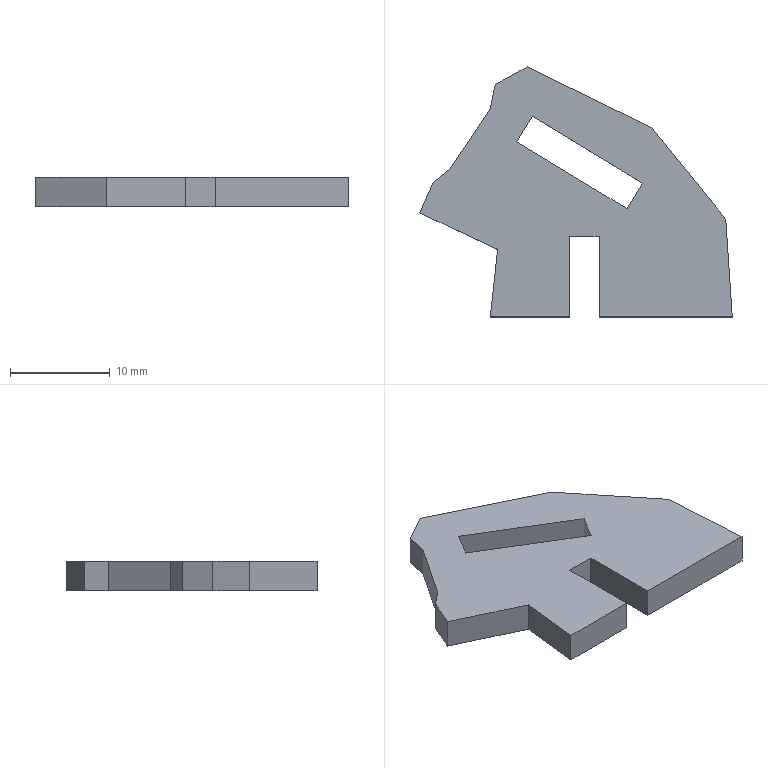Part | SolidWorks | features BaseBody 1 | 1 solid | 21 faces | box 31.393 x 25.119 x 3 mm | volume 1380 mm3 | plane 21
STEP:
#1=CARTESIAN_POINT('',(13.902,10.793,-1.5));
#2=VERTEX_POINT('',#1);
#3=CARTESIAN_POINT('',(2.824,17.525,-1.5));
#4=VERTEX_POINT('',#3);
#5=CARTESIAN_POINT('',(13.902,10.793,-1.5));
#6=DIRECTION('',(-0.8546,0.5193,0.));
#7=VECTOR('',#6,1000.);
#8=LINE('',#5,#7);
#9=EDGE_CURVE('',#2,#4,#8,.T.);
#10=ORIENTED_EDGE('',*,*,#9,.T.);
#11=CARTESIAN_POINT('',(2.824,17.525,1.5));
#12=VERTEX_POINT('',#11);
#13=CARTESIAN_POINT('',(2.824,17.525,1.5));
#14=DIRECTION('',(0.,0.,-1.));
#15=VECTOR('',#14,1000.);
#16=LINE('',#13,#15);
#17=EDGE_CURVE('',#12,#4,#16,.T.);
#18=ORIENTED_EDGE('',*,*,#17,.F.);
#19=CARTESIAN_POINT('',(13.902,10.793,1.5));
#20=VERTEX_POINT('',#19);
#21=CARTESIAN_POINT('',(13.902,10.793,1.5));
#22=DIRECTION('',(-0.8546,0.5193,0.));
#23=VECTOR('',#22,1000.);
#24=LINE('',#21,#23);
#25=EDGE_CURVE('',#20,#12,#24,.T.);
#26=ORIENTED_EDGE('',*,*,#25,.F.);
#27=CARTESIAN_POINT('',(13.902,10.793,1.5));
#28=DIRECTION('',(0.,0.,-1.));
#29=VECTOR('',#28,1000.);
#30=LINE('',#27,#29);
#31=EDGE_CURVE('',#20,#2,#30,.T.);
#32=ORIENTED_EDGE('',*,*,#31,.T.);
#33=EDGE_LOOP('',(#10,#18,#26,#32));
#34=FACE_OUTER_BOUND('',#33,.T.);
#35=CARTESIAN_POINT('',(13.902,10.793,1.5));
#36=DIRECTION('',(-0.5193,-0.8546,0.));
#37=DIRECTION('',(-0.8546,0.5193,0.));
#38=AXIS2_PLACEMENT_3D('',#35,#36,#37);
#39=PLANE('',#38);
#40=ADVANCED_FACE('',(#34),#39,.F.);
#41=CARTESIAN_POINT('',(4.382,20.086,-1.5));
#42=VERTEX_POINT('',#41);
#43=CARTESIAN_POINT('',(2.824,17.525,-1.5));
#44=DIRECTION('',(0.5198,0.8543,0.));
#45=VECTOR('',#44,1000.);
#46=LINE('',#43,#45);
#47=EDGE_CURVE('',#4,#42,#46,.T.);
#48=ORIENTED_EDGE('',*,*,#47,.T.);
#49=CARTESIAN_POINT('',(4.382,20.086,1.5));
#50=VERTEX_POINT('',#49);
#51=CARTESIAN_POINT('',(4.382,20.086,1.5));
#52=DIRECTION('',(0.,0.,-1.));
#53=VECTOR('',#52,1000.);
#54=LINE('',#51,#53);
#55=EDGE_CURVE('',#50,#42,#54,.T.);
#56=ORIENTED_EDGE('',*,*,#55,.F.);
#57=CARTESIAN_POINT('',(2.824,17.525,1.5));
#58=DIRECTION('',(0.5198,0.8543,0.));
#59=VECTOR('',#58,1000.);
#60=LINE('',#57,#59);
#61=EDGE_CURVE('',#12,#50,#60,.T.);
#62=ORIENTED_EDGE('',*,*,#61,.F.);
#63=ORIENTED_EDGE('',*,*,#17,.T.);
#64=EDGE_LOOP('',(#48,#56,#62,#63));
#65=FACE_OUTER_BOUND('',#64,.T.);
#66=CARTESIAN_POINT('',(2.824,17.525,1.5));
#67=DIRECTION('',(-0.8543,0.5198,0.));
#68=DIRECTION('',(0.,0.,1.));
#69=AXIS2_PLACEMENT_3D('',#66,#67,#68);
#70=PLANE('',#69);
#71=ADVANCED_FACE('',(#65),#70,.F.);
#72=CARTESIAN_POINT('',(15.459,13.353,-1.5));
#73=VERTEX_POINT('',#72);
#74=CARTESIAN_POINT('',(15.459,13.353,-1.5));
#75=DIRECTION('',(-0.8545,0.5194,0.));
#76=VECTOR('',#75,1000.);
#77=LINE('',#74,#76);
#78=EDGE_CURVE('',#73,#42,#77,.T.);
#79=ORIENTED_EDGE('',*,*,#78,.F.);
#80=CARTESIAN_POINT('',(15.459,13.353,1.5));
#81=VERTEX_POINT('',#80);
#82=CARTESIAN_POINT('',(15.459,13.353,1.5));
#83=DIRECTION('',(0.,0.,-1.));
#84=VECTOR('',#83,1000.);
#85=LINE('',#82,#84);
#86=EDGE_CURVE('',#81,#73,#85,.T.);
#87=ORIENTED_EDGE('',*,*,#86,.F.);
#88=CARTESIAN_POINT('',(15.459,13.353,1.5));
#89=DIRECTION('',(-0.8545,0.5194,0.));
#90=VECTOR('',#89,1000.);
#91=LINE('',#88,#90);
#92=EDGE_CURVE('',#81,#50,#91,.T.);
#93=ORIENTED_EDGE('',*,*,#92,.T.);
#94=ORIENTED_EDGE('',*,*,#55,.T.);
#95=EDGE_LOOP('',(#79,#87,#93,#94));
#96=FACE_OUTER_BOUND('',#95,.T.);
#97=CARTESIAN_POINT('',(15.459,13.353,1.5));
#98=DIRECTION('',(-0.5194,-0.8545,0.));
#99=DIRECTION('',(-0.8545,0.5194,0.));
#100=AXIS2_PLACEMENT_3D('',#97,#98,#99);
#101=PLANE('',#100);
#102=ADVANCED_FACE('',(#96),#101,.T.);
#103=CARTESIAN_POINT('',(13.902,10.793,-1.5));
#104=DIRECTION('',(0.5196,0.8544,0.));
#105=VECTOR('',#104,1000.);
#106=LINE('',#103,#105);
#107=EDGE_CURVE('',#2,#73,#106,.T.);
#108=ORIENTED_EDGE('',*,*,#107,.F.);
#109=ORIENTED_EDGE('',*,*,#31,.F.);
#110=CARTESIAN_POINT('',(13.902,10.793,1.5));
#111=DIRECTION('',(0.5196,0.8544,0.));
#112=VECTOR('',#111,1000.);
#113=LINE('',#110,#112);
#114=EDGE_CURVE('',#20,#81,#113,.T.);
#115=ORIENTED_EDGE('',*,*,#114,.T.);
#116=ORIENTED_EDGE('',*,*,#86,.T.);
#117=EDGE_LOOP('',(#108,#109,#115,#116));
#118=FACE_OUTER_BOUND('',#117,.T.);
#119=CARTESIAN_POINT('',(13.902,10.793,1.5));
#120=DIRECTION('',(-0.8544,0.5196,0.));
#121=DIRECTION('',(0.,0.,1.));
#122=AXIS2_PLACEMENT_3D('',#119,#120,#121);
#123=PLANE('',#122);
#124=ADVANCED_FACE('',(#118),#123,.T.);
#125=CARTESIAN_POINT('',(0.9023,6.7,-1.5));
#126=VERTEX_POINT('',#125);
#127=CARTESIAN_POINT('',(0.1642,-0.08325,-1.5));
#128=VERTEX_POINT('',#127);
#129=CARTESIAN_POINT('',(0.9023,6.7,-1.5));
#130=DIRECTION('',(-0.1082,-0.9941,0.));
#131=VECTOR('',#130,1000.);
#132=LINE('',#129,#131);
#133=EDGE_CURVE('',#126,#128,#132,.T.);
#134=ORIENTED_EDGE('',*,*,#133,.T.);
#135=CARTESIAN_POINT('',(0.1642,-0.08325,1.5));
#136=VERTEX_POINT('',#135);
#137=CARTESIAN_POINT('',(0.1642,-0.08325,1.5));
#138=DIRECTION('',(0.,0.,-1.));
#139=VECTOR('',#138,1000.);
#140=LINE('',#137,#139);
#141=EDGE_CURVE('',#136,#128,#140,.T.);
#142=ORIENTED_EDGE('',*,*,#141,.F.);
#143=CARTESIAN_POINT('',(0.9023,6.7,1.5));
#144=VERTEX_POINT('',#143);
#145=CARTESIAN_POINT('',(0.9023,6.7,1.5));
#146=DIRECTION('',(-0.1082,-0.9941,0.));
#147=VECTOR('',#146,1000.);
#148=LINE('',#145,#147);
#149=EDGE_CURVE('',#144,#136,#148,.T.);
#150=ORIENTED_EDGE('',*,*,#149,.F.);
#151=CARTESIAN_POINT('',(0.9023,6.7,1.5));
#152=DIRECTION('',(0.,0.,-1.));
#153=VECTOR('',#152,1000.);
#154=LINE('',#151,#153);
#155=EDGE_CURVE('',#144,#126,#154,.T.);
#156=ORIENTED_EDGE('',*,*,#155,.T.);
#157=EDGE_LOOP('',(#134,#142,#150,#156));
#158=FACE_OUTER_BOUND('',#157,.T.);
#159=CARTESIAN_POINT('',(0.9023,6.7,1.5));
#160=DIRECTION('',(0.9941,-0.1082,0.));
#161=DIRECTION('',(0.,0.,-1.));
#162=AXIS2_PLACEMENT_3D('',#159,#160,#161);
#163=PLANE('',#162);
#164=ADVANCED_FACE('',(#158),#163,.F.);
#165=CARTESIAN_POINT('',(-6.922,10.371,-1.5));
#166=VERTEX_POINT('',#165);
#167=CARTESIAN_POINT('',(-6.922,10.371,-1.5));
#168=DIRECTION('',(0.9053,-0.4248,0.));
#169=VECTOR('',#168,1000.);
#170=LINE('',#167,#169);
#171=EDGE_CURVE('',#166,#126,#170,.T.);
#172=ORIENTED_EDGE('',*,*,#171,.T.);
#173=ORIENTED_EDGE('',*,*,#155,.F.);
#174=CARTESIAN_POINT('',(-6.922,10.371,1.5));
#175=VERTEX_POINT('',#174);
#176=CARTESIAN_POINT('',(-6.922,10.371,1.5));
#177=DIRECTION('',(0.9053,-0.4248,0.));
#178=VECTOR('',#177,1000.);
#179=LINE('',#176,#178);
#180=EDGE_CURVE('',#175,#144,#179,.T.);
#181=ORIENTED_EDGE('',*,*,#180,.F.);
#182=CARTESIAN_POINT('',(-6.922,10.371,1.5));
#183=DIRECTION('',(0.,0.,-1.));
#184=VECTOR('',#183,1000.);
#185=LINE('',#182,#184);
#186=EDGE_CURVE('',#175,#166,#185,.T.);
#187=ORIENTED_EDGE('',*,*,#186,.T.);
#188=EDGE_LOOP('',(#172,#173,#181,#187));
#189=FACE_OUTER_BOUND('',#188,.T.);
#190=CARTESIAN_POINT('',(-6.922,10.371,1.5));
#191=DIRECTION('',(0.4248,0.9053,0.));
#192=DIRECTION('',(0.,0.,-1.));
#193=AXIS2_PLACEMENT_3D('',#190,#191,#192);
#194=PLANE('',#193);
#195=ADVANCED_FACE('',(#189),#194,.F.);
#196=CARTESIAN_POINT('',(-5.567,13.436,-1.5));
#197=VERTEX_POINT('',#196);
#198=CARTESIAN_POINT('',(-5.567,13.436,-1.5));
#199=DIRECTION('',(-0.4042,-0.9147,0.));
#200=VECTOR('',#199,1000.);
#201=LINE('',#198,#200);
#202=EDGE_CURVE('',#197,#166,#201,.T.);
#203=ORIENTED_EDGE('',*,*,#202,.T.);
#204=ORIENTED_EDGE('',*,*,#186,.F.);
#205=CARTESIAN_POINT('',(-5.567,13.436,1.5));
#206=VERTEX_POINT('',#205);
#207=CARTESIAN_POINT('',(-5.567,13.436,1.5));
#208=DIRECTION('',(-0.4042,-0.9147,0.));
#209=VECTOR('',#208,1000.);
#210=LINE('',#207,#209);
#211=EDGE_CURVE('',#206,#175,#210,.T.);
#212=ORIENTED_EDGE('',*,*,#211,.F.);
#213=CARTESIAN_POINT('',(-5.567,13.436,1.5));
#214=DIRECTION('',(0.,0.,-1.));
#215=VECTOR('',#214,1000.);
#216=LINE('',#213,#215);
#217=EDGE_CURVE('',#206,#197,#216,.T.);
#218=ORIENTED_EDGE('',*,*,#217,.T.);
#219=EDGE_LOOP('',(#203,#204,#212,#218));
#220=FACE_OUTER_BOUND('',#219,.T.);
#221=CARTESIAN_POINT('',(-5.567,13.436,1.5));
#222=DIRECTION('',(0.9147,-0.4042,0.));
#223=DIRECTION('',(0.,0.,-1.));
#224=AXIS2_PLACEMENT_3D('',#221,#222,#223);
#225=PLANE('',#224);
#226=ADVANCED_FACE('',(#220),#225,.F.);
#227=CARTESIAN_POINT('',(-3.99,14.678,-1.5));
#228=VERTEX_POINT('',#227);
#229=CARTESIAN_POINT('',(-3.99,14.678,-1.5));
#230=DIRECTION('',(-0.7856,-0.6187,0.));
#231=VECTOR('',#230,1000.);
#232=LINE('',#229,#231);
#233=EDGE_CURVE('',#228,#197,#232,.T.);
#234=ORIENTED_EDGE('',*,*,#233,.T.);
#235=ORIENTED_EDGE('',*,*,#217,.F.);
#236=CARTESIAN_POINT('',(-3.99,14.678,1.5));
#237=VERTEX_POINT('',#236);
#238=CARTESIAN_POINT('',(-3.99,14.678,1.5));
#239=DIRECTION('',(-0.7856,-0.6187,0.));
#240=VECTOR('',#239,1000.);
#241=LINE('',#238,#240);
#242=EDGE_CURVE('',#237,#206,#241,.T.);
#243=ORIENTED_EDGE('',*,*,#242,.F.);
#244=CARTESIAN_POINT('',(-3.99,14.678,1.5));
#245=DIRECTION('',(0.,0.,-1.));
#246=VECTOR('',#245,1000.);
#247=LINE('',#244,#246);
#248=EDGE_CURVE('',#237,#228,#247,.T.);
#249=ORIENTED_EDGE('',*,*,#248,.T.);
#250=EDGE_LOOP('',(#234,#235,#243,#249));
#251=FACE_OUTER_BOUND('',#250,.T.);
#252=CARTESIAN_POINT('',(-3.99,14.678,1.5));
#253=DIRECTION('',(0.6187,-0.7856,0.));
#254=DIRECTION('',(0.,0.,-1.));
#255=AXIS2_PLACEMENT_3D('',#252,#253,#254);
#256=PLANE('',#255);
#257=ADVANCED_FACE('',(#251),#256,.F.);
#258=CARTESIAN_POINT('',(0.1799,20.91,-1.5));
#259=VERTEX_POINT('',#258);
#260=CARTESIAN_POINT('',(0.1799,20.91,-1.5));
#261=DIRECTION('',(-0.5561,-0.8311,0.));
#262=VECTOR('',#261,1000.);
#263=LINE('',#260,#262);
#264=EDGE_CURVE('',#259,#228,#263,.T.);
#265=ORIENTED_EDGE('',*,*,#264,.T.);
#266=ORIENTED_EDGE('',*,*,#248,.F.);
#267=CARTESIAN_POINT('',(0.1799,20.91,1.5));
#268=VERTEX_POINT('',#267);
#269=CARTESIAN_POINT('',(0.1799,20.91,1.5));
#270=DIRECTION('',(-0.5561,-0.8311,0.));
#271=VECTOR('',#270,1000.);
#272=LINE('',#269,#271);
#273=EDGE_CURVE('',#268,#237,#272,.T.);
#274=ORIENTED_EDGE('',*,*,#273,.F.);
#275=CARTESIAN_POINT('',(0.1799,20.91,1.5));
#276=DIRECTION('',(0.,0.,-1.));
#277=VECTOR('',#276,1000.);
#278=LINE('',#275,#277);
#279=EDGE_CURVE('',#268,#259,#278,.T.);
#280=ORIENTED_EDGE('',*,*,#279,.T.);
#281=EDGE_LOOP('',(#265,#266,#274,#280));
#282=FACE_OUTER_BOUND('',#281,.T.);
#283=CARTESIAN_POINT('',(0.1799,20.91,1.5));
#284=DIRECTION('',(0.8311,-0.5561,0.));
#285=DIRECTION('',(0.,0.,-1.));
#286=AXIS2_PLACEMENT_3D('',#283,#284,#285);
#287=PLANE('',#286);
#288=ADVANCED_FACE('',(#282),#287,.F.);
#289=CARTESIAN_POINT('',(0.6582,23.274,-1.5));
#290=VERTEX_POINT('',#289);
#291=CARTESIAN_POINT('',(0.6582,23.274,-1.5));
#292=DIRECTION('',(-0.1984,-0.9801,0.));
#293=VECTOR('',#292,1000.);
#294=LINE('',#291,#293);
#295=EDGE_CURVE('',#290,#259,#294,.T.);
#296=ORIENTED_EDGE('',*,*,#295,.T.);
#297=ORIENTED_EDGE('',*,*,#279,.F.);
#298=CARTESIAN_POINT('',(0.6582,23.274,1.5));
#299=VERTEX_POINT('',#298);
#300=CARTESIAN_POINT('',(0.6582,23.274,1.5));
#301=DIRECTION('',(-0.1984,-0.9801,0.));
#302=VECTOR('',#301,1000.);
#303=LINE('',#300,#302);
#304=EDGE_CURVE('',#299,#268,#303,.T.);
#305=ORIENTED_EDGE('',*,*,#304,.F.);
#306=CARTESIAN_POINT('',(0.6582,23.274,1.5));
#307=DIRECTION('',(0.,0.,-1.));
#308=VECTOR('',#307,1000.);
#309=LINE('',#306,#308);
#310=EDGE_CURVE('',#299,#290,#309,.T.);
#311=ORIENTED_EDGE('',*,*,#310,.T.);
#312=EDGE_LOOP('',(#296,#297,#305,#311));
#313=FACE_OUTER_BOUND('',#312,.T.);
#314=CARTESIAN_POINT('',(0.6582,23.274,1.5));
#315=DIRECTION('',(0.9801,-0.1984,0.));
#316=DIRECTION('',(0.,0.,-1.));
#317=AXIS2_PLACEMENT_3D('',#314,#315,#316);
#318=PLANE('',#317);
#319=ADVANCED_FACE('',(#313),#318,.F.);
#320=CARTESIAN_POINT('',(3.869,25.036,-1.5));
#321=VERTEX_POINT('',#320);
#322=CARTESIAN_POINT('',(3.869,25.036,-1.5));
#323=DIRECTION('',(-0.8766,-0.4811,0.));
#324=VECTOR('',#323,1000.);
#325=LINE('',#322,#324);
#326=EDGE_CURVE('',#321,#290,#325,.T.);
#327=ORIENTED_EDGE('',*,*,#326,.T.);
#328=ORIENTED_EDGE('',*,*,#310,.F.);
#329=CARTESIAN_POINT('',(3.869,25.036,1.5));
#330=VERTEX_POINT('',#329);
#331=CARTESIAN_POINT('',(3.869,25.036,1.5));
#332=DIRECTION('',(-0.8766,-0.4811,0.));
#333=VECTOR('',#332,1000.);
#334=LINE('',#331,#333);
#335=EDGE_CURVE('',#330,#299,#334,.T.);
#336=ORIENTED_EDGE('',*,*,#335,.F.);
#337=CARTESIAN_POINT('',(3.869,25.036,1.5));
#338=DIRECTION('',(0.,0.,-1.));
#339=VECTOR('',#338,1000.);
#340=LINE('',#337,#339);
#341=EDGE_CURVE('',#330,#321,#340,.T.);
#342=ORIENTED_EDGE('',*,*,#341,.T.);
#343=EDGE_LOOP('',(#327,#328,#336,#342));
#344=FACE_OUTER_BOUND('',#343,.T.);
#345=CARTESIAN_POINT('',(3.869,25.036,1.5));
#346=DIRECTION('',(0.4811,-0.8766,0.));
#347=DIRECTION('',(0.,0.,-1.));
#348=AXIS2_PLACEMENT_3D('',#345,#346,#347);
#349=PLANE('',#348);
#350=ADVANCED_FACE('',(#344),#349,.F.);
#351=CARTESIAN_POINT('',(16.437,18.889,-1.5));
#352=VERTEX_POINT('',#351);
#353=CARTESIAN_POINT('',(16.437,18.889,-1.5));
#354=DIRECTION('',(-0.8983,0.4394,0.));
#355=VECTOR('',#354,1000.);
#356=LINE('',#353,#355);
#357=EDGE_CURVE('',#352,#321,#356,.T.);
#358=ORIENTED_EDGE('',*,*,#357,.T.);
#359=ORIENTED_EDGE('',*,*,#341,.F.);
#360=CARTESIAN_POINT('',(16.437,18.889,1.5));
#361=VERTEX_POINT('',#360);
#362=CARTESIAN_POINT('',(16.437,18.889,1.5));
#363=DIRECTION('',(-0.8983,0.4394,0.));
#364=VECTOR('',#363,1000.);
#365=LINE('',#362,#364);
#366=EDGE_CURVE('',#361,#330,#365,.T.);
#367=ORIENTED_EDGE('',*,*,#366,.F.);
#368=CARTESIAN_POINT('',(16.437,18.889,1.5));
#369=DIRECTION('',(0.,0.,-1.));
#370=VECTOR('',#369,1000.);
#371=LINE('',#368,#370);
#372=EDGE_CURVE('',#361,#352,#371,.T.);
#373=ORIENTED_EDGE('',*,*,#372,.T.);
#374=EDGE_LOOP('',(#358,#359,#367,#373));
#375=FACE_OUTER_BOUND('',#374,.T.);
#376=CARTESIAN_POINT('',(16.437,18.889,1.5));
#377=DIRECTION('',(-0.4394,-0.8983,0.));
#378=DIRECTION('',(-0.8983,0.4394,0.));
#379=AXIS2_PLACEMENT_3D('',#376,#377,#378);
#380=PLANE('',#379);
#381=ADVANCED_FACE('',(#375),#380,.F.);
#382=CARTESIAN_POINT('',(23.821,9.751,-1.5));
#383=VERTEX_POINT('',#382);
#384=CARTESIAN_POINT('',(23.821,9.751,-1.5));
#385=DIRECTION('',(-0.6285,0.7778,0.));
#386=VECTOR('',#385,1000.);
#387=LINE('',#384,#386);
#388=EDGE_CURVE('',#383,#352,#387,.T.);
#389=ORIENTED_EDGE('',*,*,#388,.T.);
#390=ORIENTED_EDGE('',*,*,#372,.F.);
#391=CARTESIAN_POINT('',(23.821,9.751,1.5));
#392=VERTEX_POINT('',#391);
#393=CARTESIAN_POINT('',(23.821,9.751,1.5));
#394=DIRECTION('',(-0.6285,0.7778,0.));
#395=VECTOR('',#394,1000.);
#396=LINE('',#393,#395);
#397=EDGE_CURVE('',#392,#361,#396,.T.);
#398=ORIENTED_EDGE('',*,*,#397,.F.);
#399=CARTESIAN_POINT('',(23.821,9.751,1.5));
#400=DIRECTION('',(0.,0.,-1.));
#401=VECTOR('',#400,1000.);
#402=LINE('',#399,#401);
#403=EDGE_CURVE('',#392,#383,#402,.T.);
#404=ORIENTED_EDGE('',*,*,#403,.T.);
#405=EDGE_LOOP('',(#389,#390,#398,#404));
#406=FACE_OUTER_BOUND('',#405,.T.);
#407=CARTESIAN_POINT('',(23.821,9.751,1.5));
#408=DIRECTION('',(-0.7778,-0.6285,0.));
#409=DIRECTION('',(-0.6285,0.7778,0.));
#410=AXIS2_PLACEMENT_3D('',#407,#408,#409);
#411=PLANE('',#410);
#412=ADVANCED_FACE('',(#406),#411,.F.);
#413=CARTESIAN_POINT('',(24.471,-0.08325,-1.5));
#414=VERTEX_POINT('',#413);
#415=CARTESIAN_POINT('',(24.471,-0.08325,-1.5));
#416=DIRECTION('',(-0.06592,0.9978,0.));
#417=VECTOR('',#416,1000.);
#418=LINE('',#415,#417);
#419=EDGE_CURVE('',#414,#383,#418,.T.);
#420=ORIENTED_EDGE('',*,*,#419,.T.);
#421=ORIENTED_EDGE('',*,*,#403,.F.);
#422=CARTESIAN_POINT('',(24.471,-0.08325,1.5));
#423=VERTEX_POINT('',#422);
#424=CARTESIAN_POINT('',(24.471,-0.08325,1.5));
#425=DIRECTION('',(-0.06592,0.9978,0.));
#426=VECTOR('',#425,1000.);
#427=LINE('',#424,#426);
#428=EDGE_CURVE('',#423,#392,#427,.T.);
#429=ORIENTED_EDGE('',*,*,#428,.F.);
#430=CARTESIAN_POINT('',(24.471,-0.08325,1.5));
#431=DIRECTION('',(0.,0.,-1.));
#432=VECTOR('',#431,1000.);
#433=LINE('',#430,#432);
#434=EDGE_CURVE('',#423,#414,#433,.T.);
#435=ORIENTED_EDGE('',*,*,#434,.T.);
#436=EDGE_LOOP('',(#420,#421,#429,#435));
#437=FACE_OUTER_BOUND('',#436,.T.);
#438=CARTESIAN_POINT('',(24.471,-0.08325,1.5));
#439=DIRECTION('',(-0.9978,-0.06592,0.));
#440=DIRECTION('',(-0.06592,0.9978,0.));
#441=AXIS2_PLACEMENT_3D('',#438,#439,#440);
#442=PLANE('',#441);
#443=ADVANCED_FACE('',(#437),#442,.F.);
#444=CARTESIAN_POINT('',(11.097,-0.08325,-1.5));
#445=VERTEX_POINT('',#444);
#446=CARTESIAN_POINT('',(24.32,-0.08325,-1.5));
#447=DIRECTION('',(1.,0.,0.));
#448=VECTOR('',#447,1000.);
#449=LINE('',#446,#448);
#450=EDGE_CURVE('',#445,#414,#449,.T.);
#451=ORIENTED_EDGE('',*,*,#450,.T.);
#452=ORIENTED_EDGE('',*,*,#434,.F.);
#453=CARTESIAN_POINT('',(11.097,-0.08325,1.5));
#454=VERTEX_POINT('',#453);
#455=CARTESIAN_POINT('',(11.097,-0.08325,1.5));
#456=DIRECTION('',(1.,0.,0.));
#457=VECTOR('',#456,1000.);
#458=LINE('',#455,#457);
#459=EDGE_CURVE('',#454,#423,#458,.T.);
#460=ORIENTED_EDGE('',*,*,#459,.F.);
#461=CARTESIAN_POINT('',(11.097,-0.08325,1.5));
#462=DIRECTION('',(0.,0.,-1.));
#463=VECTOR('',#462,1000.);
#464=LINE('',#461,#463);
#465=EDGE_CURVE('',#454,#445,#464,.T.);
#466=ORIENTED_EDGE('',*,*,#465,.T.);
#467=EDGE_LOOP('',(#451,#452,#460,#466));
#468=FACE_OUTER_BOUND('',#467,.T.);
#469=CARTESIAN_POINT('',(24.32,-0.08325,1.5));
#470=DIRECTION('',(0.,1.,0.));
#471=DIRECTION('',(1.,0.,0.));
#472=AXIS2_PLACEMENT_3D('',#469,#470,#471);
#473=PLANE('',#472);
#474=ADVANCED_FACE('',(#468),#473,.F.);
#475=CARTESIAN_POINT('',(11.097,8.001,-1.5));
#476=VERTEX_POINT('',#475);
#477=CARTESIAN_POINT('',(11.097,8.001,-1.5));
#478=DIRECTION('',(0.,-1.,0.));
#479=VECTOR('',#478,1000.);
#480=LINE('',#477,#479);
#481=EDGE_CURVE('',#476,#445,#480,.T.);
#482=ORIENTED_EDGE('',*,*,#481,.T.);
#483=ORIENTED_EDGE('',*,*,#465,.F.);
#484=CARTESIAN_POINT('',(11.097,8.001,1.5));
#485=VERTEX_POINT('',#484);
#486=CARTESIAN_POINT('',(11.097,8.001,1.5));
#487=DIRECTION('',(0.,-1.,0.));
#488=VECTOR('',#487,1000.);
#489=LINE('',#486,#488);
#490=EDGE_CURVE('',#485,#454,#489,.T.);
#491=ORIENTED_EDGE('',*,*,#490,.F.);
#492=CARTESIAN_POINT('',(11.097,8.001,1.5));
#493=DIRECTION('',(0.,0.,-1.));
#494=VECTOR('',#493,1000.);
#495=LINE('',#492,#494);
#496=EDGE_CURVE('',#485,#476,#495,.T.);
#497=ORIENTED_EDGE('',*,*,#496,.T.);
#498=EDGE_LOOP('',(#482,#483,#491,#497));
#499=FACE_OUTER_BOUND('',#498,.T.);
#500=CARTESIAN_POINT('',(11.097,8.001,1.5));
#501=DIRECTION('',(1.,0.,0.));
#502=DIRECTION('',(0.,1.,0.));
#503=AXIS2_PLACEMENT_3D('',#500,#501,#502);
#504=PLANE('',#503);
#505=ADVANCED_FACE('',(#499),#504,.F.);
#506=CARTESIAN_POINT('',(8.101,8.001,-1.5));
#507=VERTEX_POINT('',#506);
#508=CARTESIAN_POINT('',(8.101,8.001,-1.5));
#509=DIRECTION('',(1.,0.,0.));
#510=VECTOR('',#509,1000.);
#511=LINE('',#508,#510);
#512=EDGE_CURVE('',#507,#476,#511,.T.);
#513=ORIENTED_EDGE('',*,*,#512,.T.);
#514=ORIENTED_EDGE('',*,*,#496,.F.);
#515=CARTESIAN_POINT('',(8.101,8.001,1.5));
#516=VERTEX_POINT('',#515);
#517=CARTESIAN_POINT('',(8.101,8.001,1.5));
#518=DIRECTION('',(1.,0.,0.));
#519=VECTOR('',#518,1000.);
#520=LINE('',#517,#519);
#521=EDGE_CURVE('',#516,#485,#520,.T.);
#522=ORIENTED_EDGE('',*,*,#521,.F.);
#523=CARTESIAN_POINT('',(8.101,8.001,1.5));
#524=DIRECTION('',(0.,0.,-1.));
#525=VECTOR('',#524,1000.);
#526=LINE('',#523,#525);
#527=EDGE_CURVE('',#516,#507,#526,.T.);
#528=ORIENTED_EDGE('',*,*,#527,.T.);
#529=EDGE_LOOP('',(#513,#514,#522,#528));
#530=FACE_OUTER_BOUND('',#529,.T.);
#531=CARTESIAN_POINT('',(8.101,8.001,1.5));
#532=DIRECTION('',(0.,1.,0.));
#533=DIRECTION('',(1.,0.,0.));
#534=AXIS2_PLACEMENT_3D('',#531,#532,#533);
#535=PLANE('',#534);
#536=ADVANCED_FACE('',(#530),#535,.F.);
#537=CARTESIAN_POINT('',(8.101,-0.08325,-1.5));
#538=VERTEX_POINT('',#537);
#539=CARTESIAN_POINT('',(8.101,-0.08325,-1.5));
#540=DIRECTION('',(0.,1.,0.));
#541=VECTOR('',#540,1000.);
#542=LINE('',#539,#541);
#543=EDGE_CURVE('',#538,#507,#542,.T.);
#544=ORIENTED_EDGE('',*,*,#543,.T.);
#545=ORIENTED_EDGE('',*,*,#527,.F.);
#546=CARTESIAN_POINT('',(8.101,-0.08325,1.5));
#547=VERTEX_POINT('',#546);
#548=CARTESIAN_POINT('',(8.101,-0.08325,1.5));
#549=DIRECTION('',(0.,1.,0.));
#550=VECTOR('',#549,1000.);
#551=LINE('',#548,#550);
#552=EDGE_CURVE('',#547,#516,#551,.T.);
#553=ORIENTED_EDGE('',*,*,#552,.F.);
#554=CARTESIAN_POINT('',(8.101,-0.08325,1.5));
#555=DIRECTION('',(0.,0.,-1.));
#556=VECTOR('',#555,1000.);
#557=LINE('',#554,#556);
#558=EDGE_CURVE('',#547,#538,#557,.T.);
#559=ORIENTED_EDGE('',*,*,#558,.T.);
#560=EDGE_LOOP('',(#544,#545,#553,#559));
#561=FACE_OUTER_BOUND('',#560,.T.);
#562=CARTESIAN_POINT('',(8.101,-0.08325,1.5));
#563=DIRECTION('',(-1.,0.,0.));
#564=DIRECTION('',(0.,0.,1.));
#565=AXIS2_PLACEMENT_3D('',#562,#563,#564);
#566=PLANE('',#565);
#567=ADVANCED_FACE('',(#561),#566,.F.);
#568=CARTESIAN_POINT('',(0.1642,-0.08325,-1.5));
#569=DIRECTION('',(1.,0.,0.));
#570=VECTOR('',#569,1000.);
#571=LINE('',#568,#570);
#572=EDGE_CURVE('',#128,#538,#571,.T.);
#573=ORIENTED_EDGE('',*,*,#572,.T.);
#574=ORIENTED_EDGE('',*,*,#558,.F.);
#575=CARTESIAN_POINT('',(0.1642,-0.08325,1.5));
#576=DIRECTION('',(1.,0.,0.));
#577=VECTOR('',#576,1000.);
#578=LINE('',#575,#577);
#579=EDGE_CURVE('',#136,#547,#578,.T.);
#580=ORIENTED_EDGE('',*,*,#579,.F.);
#581=ORIENTED_EDGE('',*,*,#141,.T.);
#582=EDGE_LOOP('',(#573,#574,#580,#581));
#583=FACE_OUTER_BOUND('',#582,.T.);
#584=CARTESIAN_POINT('',(0.1642,-0.08325,1.5));
#585=DIRECTION('',(0.,1.,0.));
#586=DIRECTION('',(1.,0.,0.));
#587=AXIS2_PLACEMENT_3D('',#584,#585,#586);
#588=PLANE('',#587);
#589=ADVANCED_FACE('',(#583),#588,.F.);
#590=ORIENTED_EDGE('',*,*,#107,.T.);
#591=ORIENTED_EDGE('',*,*,#78,.T.);
#592=ORIENTED_EDGE('',*,*,#47,.F.);
#593=ORIENTED_EDGE('',*,*,#9,.F.);
#594=EDGE_LOOP('',(#590,#591,#592,#593));
#595=FACE_BOUND('',#594,.T.);
#596=ORIENTED_EDGE('',*,*,#572,.F.);
#597=ORIENTED_EDGE('',*,*,#133,.F.);
#598=ORIENTED_EDGE('',*,*,#171,.F.);
#599=ORIENTED_EDGE('',*,*,#202,.F.);
#600=ORIENTED_EDGE('',*,*,#233,.F.);
#601=ORIENTED_EDGE('',*,*,#264,.F.);
#602=ORIENTED_EDGE('',*,*,#295,.F.);
#603=ORIENTED_EDGE('',*,*,#326,.F.);
#604=ORIENTED_EDGE('',*,*,#357,.F.);
#605=ORIENTED_EDGE('',*,*,#388,.F.);
#606=ORIENTED_EDGE('',*,*,#419,.F.);
#607=ORIENTED_EDGE('',*,*,#450,.F.);
#608=ORIENTED_EDGE('',*,*,#481,.F.);
#609=ORIENTED_EDGE('',*,*,#512,.F.);
#610=ORIENTED_EDGE('',*,*,#543,.F.);
#611=EDGE_LOOP('',(#596,#597,#598,#599,#600,#601,#602,#603,#604,#605,#606,#607,#608,#609,#610));
#612=FACE_OUTER_BOUND('',#611,.T.);
#613=CARTESIAN_POINT('',(0.,0.,-1.5));
#614=DIRECTION('',(0.,0.,1.));
#615=DIRECTION('',(1.,0.,0.));
#616=AXIS2_PLACEMENT_3D('',#613,#614,#615);
#617=PLANE('',#616);
#618=ADVANCED_FACE('',(#595,#612),#617,.F.);
#619=ORIENTED_EDGE('',*,*,#92,.F.);
#620=ORIENTED_EDGE('',*,*,#114,.F.);
#621=ORIENTED_EDGE('',*,*,#25,.T.);
#622=ORIENTED_EDGE('',*,*,#61,.T.);
#623=EDGE_LOOP('',(#619,#620,#621,#622));
#624=FACE_BOUND('',#623,.T.);
#625=ORIENTED_EDGE('',*,*,#579,.T.);
#626=ORIENTED_EDGE('',*,*,#552,.T.);
#627=ORIENTED_EDGE('',*,*,#521,.T.);
#628=ORIENTED_EDGE('',*,*,#490,.T.);
#629=ORIENTED_EDGE('',*,*,#459,.T.);
#630=ORIENTED_EDGE('',*,*,#428,.T.);
#631=ORIENTED_EDGE('',*,*,#397,.T.);
#632=ORIENTED_EDGE('',*,*,#366,.T.);
#633=ORIENTED_EDGE('',*,*,#335,.T.);
#634=ORIENTED_EDGE('',*,*,#304,.T.);
#635=ORIENTED_EDGE('',*,*,#273,.T.);
#636=ORIENTED_EDGE('',*,*,#242,.T.);
#637=ORIENTED_EDGE('',*,*,#211,.T.);
#638=ORIENTED_EDGE('',*,*,#180,.T.);
#639=ORIENTED_EDGE('',*,*,#149,.T.);
#640=EDGE_LOOP('',(#625,#626,#627,#628,#629,#630,#631,#632,#633,#634,#635,#636,#637,#638,#639));
#641=FACE_OUTER_BOUND('',#640,.T.);
#642=CARTESIAN_POINT('',(0.,0.,1.5));
#643=DIRECTION('',(0.,0.,1.));
#644=DIRECTION('',(1.,0.,0.));
#645=AXIS2_PLACEMENT_3D('',#642,#643,#644);
#646=PLANE('',#645);
#647=ADVANCED_FACE('',(#624,#641),#646,.T.);
#648=CLOSED_SHELL('',(#40,#71,#102,#124,#164,#195,#226,#257,#288,#319,#350,#381,#412,#443,#474,#505,#536,#567,#589,#618,#647));
#649=MANIFOLD_SOLID_BREP('',#648);
#650=CARTESIAN_POINT('',(0.,0.,0.));
#651=DIRECTION('',(0.,0.,1.));
#652=DIRECTION('',(1.,0.,0.));
#653=AXIS2_PLACEMENT_3D('',#650,#651,#652);
#654=(LENGTH_UNIT()NAMED_UNIT(*)SI_UNIT(.MILLI.,.METRE.));
#655=UNCERTAINTY_MEASURE_WITH_UNIT(LENGTH_MEASURE(0.00001),#654,'','');
#656=(NAMED_UNIT(*)PLANE_ANGLE_UNIT()SI_UNIT($,.RADIAN.));
#657=(NAMED_UNIT(*)SI_UNIT($,.STERADIAN.)SOLID_ANGLE_UNIT());
#658=(GEOMETRIC_REPRESENTATION_CONTEXT(3)GLOBAL_UNCERTAINTY_ASSIGNED_CONTEXT((#655))GLOBAL_UNIT_ASSIGNED_CONTEXT((#654,#656,#657))REPRESENTATION_CONTEXT('',''));
#659=ADVANCED_BREP_SHAPE_REPRESENTATION('',(#649,#653),#658);